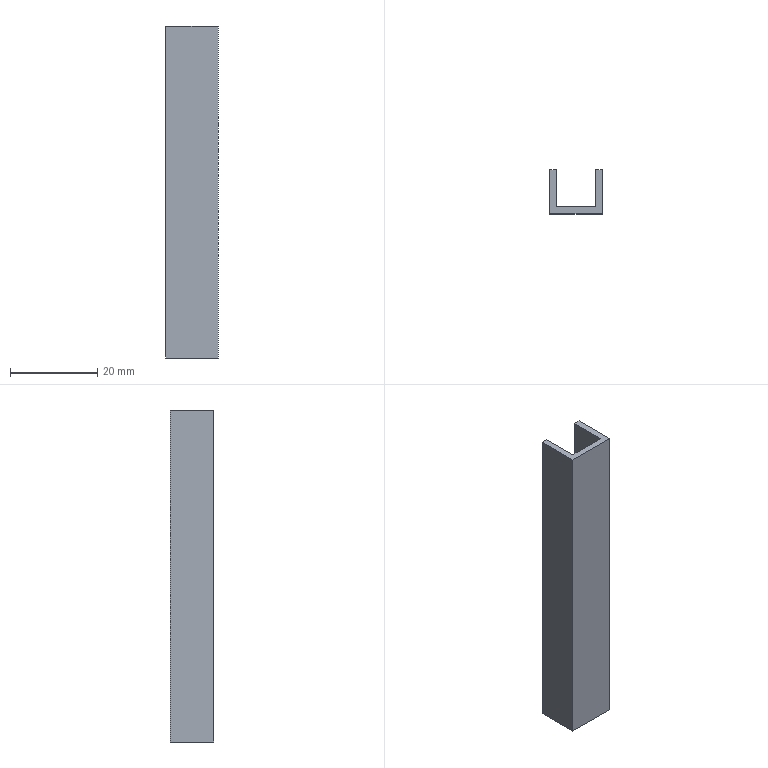Part | SolidWorks | features Extrusion 1, ICE 1 | 1 solid | 10 faces | box 12 x 10 x 76 mm | volume 3306 mm3 | plane 10
STEP:
#1=CARTESIAN_POINT('',(-6.,5.,31.));
#2=VERTEX_POINT('',#1);
#3=CARTESIAN_POINT('',(-6.,-5.,31.));
#4=VERTEX_POINT('',#3);
#5=CARTESIAN_POINT('',(-6.,5.,31.));
#6=DIRECTION('',(0.,-1.,0.));
#7=VECTOR('',#6,1000.);
#8=LINE('',#5,#7);
#9=EDGE_CURVE('',#2,#4,#8,.T.);
#10=ORIENTED_EDGE('',*,*,#9,.F.);
#11=CARTESIAN_POINT('',(-6.,5.,-45.));
#12=VERTEX_POINT('',#11);
#13=CARTESIAN_POINT('',(-6.,5.,-45.));
#14=DIRECTION('',(0.,0.,1.));
#15=VECTOR('',#14,1000.);
#16=LINE('',#13,#15);
#17=EDGE_CURVE('',#12,#2,#16,.T.);
#18=ORIENTED_EDGE('',*,*,#17,.F.);
#19=CARTESIAN_POINT('',(-6.,-5.,-45.));
#20=VERTEX_POINT('',#19);
#21=CARTESIAN_POINT('',(-6.,5.,-45.));
#22=DIRECTION('',(0.,-1.,0.));
#23=VECTOR('',#22,1000.);
#24=LINE('',#21,#23);
#25=EDGE_CURVE('',#12,#20,#24,.T.);
#26=ORIENTED_EDGE('',*,*,#25,.T.);
#27=CARTESIAN_POINT('',(-6.,-5.,-45.));
#28=DIRECTION('',(0.,0.,1.));
#29=VECTOR('',#28,1000.);
#30=LINE('',#27,#29);
#31=EDGE_CURVE('',#20,#4,#30,.T.);
#32=ORIENTED_EDGE('',*,*,#31,.T.);
#33=EDGE_LOOP('',(#10,#18,#26,#32));
#34=FACE_OUTER_BOUND('',#33,.T.);
#35=CARTESIAN_POINT('',(-6.,5.,-45.));
#36=DIRECTION('',(-1.,0.,0.));
#37=DIRECTION('',(0.,0.,1.));
#38=AXIS2_PLACEMENT_3D('',#35,#36,#37);
#39=PLANE('',#38);
#40=ADVANCED_FACE('',(#34),#39,.T.);
#41=CARTESIAN_POINT('',(-4.5,5.,31.));
#42=VERTEX_POINT('',#41);
#43=CARTESIAN_POINT('',(-4.5,5.,31.));
#44=DIRECTION('',(-1.,0.,0.));
#45=VECTOR('',#44,1000.);
#46=LINE('',#43,#45);
#47=EDGE_CURVE('',#42,#2,#46,.T.);
#48=ORIENTED_EDGE('',*,*,#47,.F.);
#49=CARTESIAN_POINT('',(-4.5,5.,-45.));
#50=VERTEX_POINT('',#49);
#51=CARTESIAN_POINT('',(-4.5,5.,-45.));
#52=DIRECTION('',(0.,0.,1.));
#53=VECTOR('',#52,1000.);
#54=LINE('',#51,#53);
#55=EDGE_CURVE('',#50,#42,#54,.T.);
#56=ORIENTED_EDGE('',*,*,#55,.F.);
#57=CARTESIAN_POINT('',(-4.5,5.,-45.));
#58=DIRECTION('',(-1.,0.,0.));
#59=VECTOR('',#58,1000.);
#60=LINE('',#57,#59);
#61=EDGE_CURVE('',#50,#12,#60,.T.);
#62=ORIENTED_EDGE('',*,*,#61,.T.);
#63=ORIENTED_EDGE('',*,*,#17,.T.);
#64=EDGE_LOOP('',(#48,#56,#62,#63));
#65=FACE_OUTER_BOUND('',#64,.T.);
#66=CARTESIAN_POINT('',(-4.5,5.,-45.));
#67=DIRECTION('',(0.,1.,0.));
#68=DIRECTION('',(0.,0.,1.));
#69=AXIS2_PLACEMENT_3D('',#66,#67,#68);
#70=PLANE('',#69);
#71=ADVANCED_FACE('',(#65),#70,.T.);
#72=CARTESIAN_POINT('',(-4.5,-3.5,31.));
#73=VERTEX_POINT('',#72);
#74=CARTESIAN_POINT('',(-4.5,-3.5,31.));
#75=DIRECTION('',(0.,1.,0.));
#76=VECTOR('',#75,1000.);
#77=LINE('',#74,#76);
#78=EDGE_CURVE('',#73,#42,#77,.T.);
#79=ORIENTED_EDGE('',*,*,#78,.F.);
#80=CARTESIAN_POINT('',(-4.5,-3.5,-45.));
#81=VERTEX_POINT('',#80);
#82=CARTESIAN_POINT('',(-4.5,-3.5,-45.));
#83=DIRECTION('',(0.,0.,1.));
#84=VECTOR('',#83,1000.);
#85=LINE('',#82,#84);
#86=EDGE_CURVE('',#81,#73,#85,.T.);
#87=ORIENTED_EDGE('',*,*,#86,.F.);
#88=CARTESIAN_POINT('',(-4.5,-3.5,-45.));
#89=DIRECTION('',(0.,1.,0.));
#90=VECTOR('',#89,1000.);
#91=LINE('',#88,#90);
#92=EDGE_CURVE('',#81,#50,#91,.T.);
#93=ORIENTED_EDGE('',*,*,#92,.T.);
#94=ORIENTED_EDGE('',*,*,#55,.T.);
#95=EDGE_LOOP('',(#79,#87,#93,#94));
#96=FACE_OUTER_BOUND('',#95,.T.);
#97=CARTESIAN_POINT('',(-4.5,-3.5,-45.));
#98=DIRECTION('',(1.,0.,0.));
#99=DIRECTION('',(0.,0.,-1.));
#100=AXIS2_PLACEMENT_3D('',#97,#98,#99);
#101=PLANE('',#100);
#102=ADVANCED_FACE('',(#96),#101,.T.);
#103=CARTESIAN_POINT('',(4.5,-3.5,31.));
#104=VERTEX_POINT('',#103);
#105=CARTESIAN_POINT('',(4.5,-3.5,31.));
#106=DIRECTION('',(-1.,0.,0.));
#107=VECTOR('',#106,1000.);
#108=LINE('',#105,#107);
#109=EDGE_CURVE('',#104,#73,#108,.T.);
#110=ORIENTED_EDGE('',*,*,#109,.F.);
#111=CARTESIAN_POINT('',(4.5,-3.5,-45.));
#112=VERTEX_POINT('',#111);
#113=CARTESIAN_POINT('',(4.5,-3.5,-45.));
#114=DIRECTION('',(0.,0.,1.));
#115=VECTOR('',#114,1000.);
#116=LINE('',#113,#115);
#117=EDGE_CURVE('',#112,#104,#116,.T.);
#118=ORIENTED_EDGE('',*,*,#117,.F.);
#119=CARTESIAN_POINT('',(4.5,-3.5,-45.));
#120=DIRECTION('',(-1.,0.,0.));
#121=VECTOR('',#120,1000.);
#122=LINE('',#119,#121);
#123=EDGE_CURVE('',#112,#81,#122,.T.);
#124=ORIENTED_EDGE('',*,*,#123,.T.);
#125=ORIENTED_EDGE('',*,*,#86,.T.);
#126=EDGE_LOOP('',(#110,#118,#124,#125));
#127=FACE_OUTER_BOUND('',#126,.T.);
#128=CARTESIAN_POINT('',(4.5,-3.5,-45.));
#129=DIRECTION('',(0.,1.,0.));
#130=DIRECTION('',(0.,0.,1.));
#131=AXIS2_PLACEMENT_3D('',#128,#129,#130);
#132=PLANE('',#131);
#133=ADVANCED_FACE('',(#127),#132,.T.);
#134=CARTESIAN_POINT('',(4.5,5.,31.));
#135=VERTEX_POINT('',#134);
#136=CARTESIAN_POINT('',(4.5,5.,31.));
#137=DIRECTION('',(0.,-1.,0.));
#138=VECTOR('',#137,1000.);
#139=LINE('',#136,#138);
#140=EDGE_CURVE('',#135,#104,#139,.T.);
#141=ORIENTED_EDGE('',*,*,#140,.F.);
#142=CARTESIAN_POINT('',(4.5,5.,-45.));
#143=VERTEX_POINT('',#142);
#144=CARTESIAN_POINT('',(4.5,5.,-45.));
#145=DIRECTION('',(0.,0.,1.));
#146=VECTOR('',#145,1000.);
#147=LINE('',#144,#146);
#148=EDGE_CURVE('',#143,#135,#147,.T.);
#149=ORIENTED_EDGE('',*,*,#148,.F.);
#150=CARTESIAN_POINT('',(4.5,5.,-45.));
#151=DIRECTION('',(0.,-1.,0.));
#152=VECTOR('',#151,1000.);
#153=LINE('',#150,#152);
#154=EDGE_CURVE('',#143,#112,#153,.T.);
#155=ORIENTED_EDGE('',*,*,#154,.T.);
#156=ORIENTED_EDGE('',*,*,#117,.T.);
#157=EDGE_LOOP('',(#141,#149,#155,#156));
#158=FACE_OUTER_BOUND('',#157,.T.);
#159=CARTESIAN_POINT('',(4.5,5.,-45.));
#160=DIRECTION('',(-1.,0.,0.));
#161=DIRECTION('',(0.,0.,1.));
#162=AXIS2_PLACEMENT_3D('',#159,#160,#161);
#163=PLANE('',#162);
#164=ADVANCED_FACE('',(#158),#163,.T.);
#165=CARTESIAN_POINT('',(6.,5.,31.));
#166=VERTEX_POINT('',#165);
#167=CARTESIAN_POINT('',(6.,5.,31.));
#168=DIRECTION('',(-1.,0.,0.));
#169=VECTOR('',#168,1000.);
#170=LINE('',#167,#169);
#171=EDGE_CURVE('',#166,#135,#170,.T.);
#172=ORIENTED_EDGE('',*,*,#171,.F.);
#173=CARTESIAN_POINT('',(6.,5.,-45.));
#174=VERTEX_POINT('',#173);
#175=CARTESIAN_POINT('',(6.,5.,-45.));
#176=DIRECTION('',(0.,0.,1.));
#177=VECTOR('',#176,1000.);
#178=LINE('',#175,#177);
#179=EDGE_CURVE('',#174,#166,#178,.T.);
#180=ORIENTED_EDGE('',*,*,#179,.F.);
#181=CARTESIAN_POINT('',(6.,5.,-45.));
#182=DIRECTION('',(-1.,0.,0.));
#183=VECTOR('',#182,1000.);
#184=LINE('',#181,#183);
#185=EDGE_CURVE('',#174,#143,#184,.T.);
#186=ORIENTED_EDGE('',*,*,#185,.T.);
#187=ORIENTED_EDGE('',*,*,#148,.T.);
#188=EDGE_LOOP('',(#172,#180,#186,#187));
#189=FACE_OUTER_BOUND('',#188,.T.);
#190=CARTESIAN_POINT('',(6.,5.,-45.));
#191=DIRECTION('',(0.,1.,0.));
#192=DIRECTION('',(0.,0.,1.));
#193=AXIS2_PLACEMENT_3D('',#190,#191,#192);
#194=PLANE('',#193);
#195=ADVANCED_FACE('',(#189),#194,.T.);
#196=CARTESIAN_POINT('',(6.,-5.,31.));
#197=VERTEX_POINT('',#196);
#198=CARTESIAN_POINT('',(6.,-5.,31.));
#199=DIRECTION('',(0.,1.,0.));
#200=VECTOR('',#199,1000.);
#201=LINE('',#198,#200);
#202=EDGE_CURVE('',#197,#166,#201,.T.);
#203=ORIENTED_EDGE('',*,*,#202,.F.);
#204=CARTESIAN_POINT('',(6.,-5.,-45.));
#205=VERTEX_POINT('',#204);
#206=CARTESIAN_POINT('',(6.,-5.,-45.));
#207=DIRECTION('',(0.,0.,1.));
#208=VECTOR('',#207,1000.);
#209=LINE('',#206,#208);
#210=EDGE_CURVE('',#205,#197,#209,.T.);
#211=ORIENTED_EDGE('',*,*,#210,.F.);
#212=CARTESIAN_POINT('',(6.,-5.,-45.));
#213=DIRECTION('',(0.,1.,0.));
#214=VECTOR('',#213,1000.);
#215=LINE('',#212,#214);
#216=EDGE_CURVE('',#205,#174,#215,.T.);
#217=ORIENTED_EDGE('',*,*,#216,.T.);
#218=ORIENTED_EDGE('',*,*,#179,.T.);
#219=EDGE_LOOP('',(#203,#211,#217,#218));
#220=FACE_OUTER_BOUND('',#219,.T.);
#221=CARTESIAN_POINT('',(6.,-5.,-45.));
#222=DIRECTION('',(1.,0.,0.));
#223=DIRECTION('',(0.,0.,-1.));
#224=AXIS2_PLACEMENT_3D('',#221,#222,#223);
#225=PLANE('',#224);
#226=ADVANCED_FACE('',(#220),#225,.T.);
#227=CARTESIAN_POINT('',(-6.,-5.,31.));
#228=DIRECTION('',(1.,0.,0.));
#229=VECTOR('',#228,1000.);
#230=LINE('',#227,#229);
#231=EDGE_CURVE('',#4,#197,#230,.T.);
#232=ORIENTED_EDGE('',*,*,#231,.F.);
#233=ORIENTED_EDGE('',*,*,#31,.F.);
#234=CARTESIAN_POINT('',(-6.,-5.,-45.));
#235=DIRECTION('',(1.,0.,0.));
#236=VECTOR('',#235,1000.);
#237=LINE('',#234,#236);
#238=EDGE_CURVE('',#20,#205,#237,.T.);
#239=ORIENTED_EDGE('',*,*,#238,.T.);
#240=ORIENTED_EDGE('',*,*,#210,.T.);
#241=EDGE_LOOP('',(#232,#233,#239,#240));
#242=FACE_OUTER_BOUND('',#241,.T.);
#243=CARTESIAN_POINT('',(-6.,-5.,-45.));
#244=DIRECTION('',(0.,-1.,0.));
#245=DIRECTION('',(0.,0.,-1.));
#246=AXIS2_PLACEMENT_3D('',#243,#244,#245);
#247=PLANE('',#246);
#248=ADVANCED_FACE('',(#242),#247,.T.);
#249=ORIENTED_EDGE('',*,*,#25,.F.);
#250=ORIENTED_EDGE('',*,*,#61,.F.);
#251=ORIENTED_EDGE('',*,*,#92,.F.);
#252=ORIENTED_EDGE('',*,*,#123,.F.);
#253=ORIENTED_EDGE('',*,*,#154,.F.);
#254=ORIENTED_EDGE('',*,*,#185,.F.);
#255=ORIENTED_EDGE('',*,*,#216,.F.);
#256=ORIENTED_EDGE('',*,*,#238,.F.);
#257=EDGE_LOOP('',(#249,#250,#251,#252,#253,#254,#255,#256));
#258=FACE_OUTER_BOUND('',#257,.T.);
#259=CARTESIAN_POINT('',(0.,0.,-45.));
#260=DIRECTION('',(0.,0.,1.));
#261=DIRECTION('',(1.,0.,0.));
#262=AXIS2_PLACEMENT_3D('',#259,#260,#261);
#263=PLANE('',#262);
#264=ADVANCED_FACE('',(#258),#263,.F.);
#265=ORIENTED_EDGE('',*,*,#9,.T.);
#266=ORIENTED_EDGE('',*,*,#231,.T.);
#267=ORIENTED_EDGE('',*,*,#202,.T.);
#268=ORIENTED_EDGE('',*,*,#171,.T.);
#269=ORIENTED_EDGE('',*,*,#140,.T.);
#270=ORIENTED_EDGE('',*,*,#109,.T.);
#271=ORIENTED_EDGE('',*,*,#78,.T.);
#272=ORIENTED_EDGE('',*,*,#47,.T.);
#273=EDGE_LOOP('',(#265,#266,#267,#268,#269,#270,#271,#272));
#274=FACE_OUTER_BOUND('',#273,.T.);
#275=CARTESIAN_POINT('',(-10.,-6.,31.));
#276=DIRECTION('',(0.,0.,-1.));
#277=DIRECTION('',(-1.,0.,0.));
#278=AXIS2_PLACEMENT_3D('',#275,#276,#277);
#279=PLANE('',#278);
#280=ADVANCED_FACE('',(#274),#279,.F.);
#281=CLOSED_SHELL('',(#40,#71,#102,#133,#164,#195,#226,#248,#264,#280));
#282=MANIFOLD_SOLID_BREP('',#281);
#283=CARTESIAN_POINT('',(0.,0.,0.));
#284=DIRECTION('',(0.,0.,1.));
#285=DIRECTION('',(1.,0.,0.));
#286=AXIS2_PLACEMENT_3D('',#283,#284,#285);
#287=(LENGTH_UNIT()NAMED_UNIT(*)SI_UNIT(.MILLI.,.METRE.));
#288=UNCERTAINTY_MEASURE_WITH_UNIT(LENGTH_MEASURE(0.00001),#287,'','');
#289=(NAMED_UNIT(*)PLANE_ANGLE_UNIT()SI_UNIT($,.RADIAN.));
#290=(NAMED_UNIT(*)SI_UNIT($,.STERADIAN.)SOLID_ANGLE_UNIT());
#291=(GEOMETRIC_REPRESENTATION_CONTEXT(3)GLOBAL_UNCERTAINTY_ASSIGNED_CONTEXT((#288))GLOBAL_UNIT_ASSIGNED_CONTEXT((#287,#289,#290))REPRESENTATION_CONTEXT('',''));
#292=ADVANCED_BREP_SHAPE_REPRESENTATION('',(#282,#286),#291);